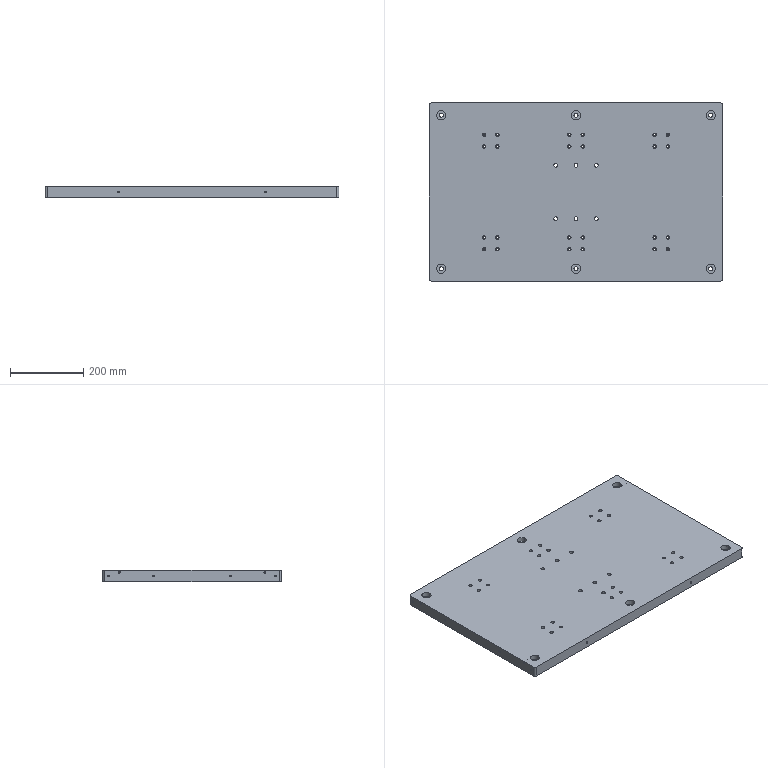NC program | Mastercam | posted with a generic post | part box 800 x 485 x 30 mm
Lines 983 to 1630 of 7047:
N9750 T5 M6
N9760 G0 G90 G17 G54 X250. Y-156. A0. S6500 M3
N9770 G43 H5 Z50. M8
N9780 Z1.
N9790 G1 Z0. F600.
N9800 X250.955 Y-155.045 F2000.
N9810 G3 X250. Y-154.09 I-.955 J0.
N9820 X248.09 Y-156. Z-.125 I0. J-1.91
N9830 X250. Y-157.91 Z-.25 I1.91 J0.
N9840 X251.91 Y-156. Z-.375 I0. J1.91
N9850 X250. Y-154.09 Z-.5 I-1.91 J0.
N9860 X248.09 Y-156. Z-.625 I0. J-1.91
N9870 X250. Y-157.91 Z-.75 I1.91 J0.
N9880 X251.91 Y-156. Z-.875 I0. J1.91
N9890 X250. Y-154.09 Z-1. I-1.91 J0.
N9900 X248.09 Y-156. Z-1.125 I0. J-1.91
N9910 X250. Y-157.91 Z-1.25 I1.91 J0.
N9920 X251.91 Y-156. Z-1.375 I0. J1.91
N9930 X250. Y-154.09 Z-1.5 I-1.91 J0.
N9940 X248.09 Y-156. Z-1.625 I0. J-1.91
N9950 X250. Y-157.91 Z-1.75 I1.91 J0.
N9960 X251.91 Y-156. Z-1.875 I0. J1.91
N9970 X250. Y-154.09 Z-2. I-1.91 J0.
N9980 X248.09 Y-156. Z-2.125 I0. J-1.91
N9990 X250. Y-157.91 Z-2.25 I1.91 J0.
N100 X251.91 Y-156. Z-2.375 I0. J1.91
N110 X250. Y-154.09 Z-2.5 I-1.91 J0.
N120 X248.09 Y-156. Z-2.625 I0. J-1.91
N130 X250. Y-157.91 Z-2.75 I1.91 J0.
N140 X251.91 Y-156. Z-2.875 I0. J1.91
N150 X250. Y-154.09 Z-3. I-1.91 J0.
N160 X248.09 Y-156. Z-3.125 I0. J-1.91
N170 X250. Y-157.91 Z-3.25 I1.91 J0.
N180 X251.91 Y-156. Z-3.375 I0. J1.91
N190 X250. Y-154.09 Z-3.5 I-1.91 J0.
N200 X248.09 Y-156. Z-3.625 I0. J-1.91
N210 X250. Y-157.91 Z-3.75 I1.91 J0.
N220 X251.91 Y-156. Z-3.875 I0. J1.91
N230 X250. Y-154.09 Z-4. I-1.91 J0.
N240 X248.09 Y-156. Z-4.125 I0. J-1.91
N250 X250. Y-157.91 Z-4.25 I1.91 J0.
N260 X251.91 Y-156. Z-4.375 I0. J1.91
N270 X250. Y-154.09 Z-4.5 I-1.91 J0.
N280 X248.09 Y-156. Z-4.625 I0. J-1.91
N290 X250. Y-157.91 Z-4.75 I1.91 J0.
N300 X251.91 Y-156. Z-4.875 I0. J1.91
N310 X250. Y-154.09 Z-5. I-1.91 J0.
N320 X248.09 Y-156. Z-5.125 I0. J-1.91
N330 X250. Y-157.91 Z-5.25 I1.91 J0.
N340 X251.91 Y-156. Z-5.375 I0. J1.91
N350 X250. Y-154.09 Z-5.5 I-1.91 J0.
N360 X248.09 Y-156. Z-5.625 I0. J-1.91
N370 X250. Y-157.91 Z-5.75 I1.91 J0.
N380 X251.91 Y-156. Z-5.875 I0. J1.91
N390 X250. Y-154.09 Z-6. I-1.91 J0.
N400 X248.09 Y-156. Z-6.125 I0. J-1.91
N410 X250. Y-157.91 Z-6.25 I1.91 J0.
N420 X251.91 Y-156. Z-6.375 I0. J1.91
N430 X250. Y-154.09 Z-6.5 I-1.91 J0.
N440 X248.09 Y-156. Z-6.625 I0. J-1.91
N450 X250. Y-157.91 Z-6.75 I1.91 J0.
N460 X251.91 Y-156. Z-6.875 I0. J1.91
N470 X250. Y-154.09 Z-7. I-1.91 J0.
N480 X248.09 Y-156. Z-7.125 I0. J-1.91
N490 X250. Y-157.91 Z-7.25 I1.91 J0.
N500 X251.91 Y-156. Z-7.375 I0. J1.91
N510 X250. Y-154.09 Z-7.5 I-1.91 J0.
N520 X248.09 Y-156. Z-7.625 I0. J-1.91
N530 X250. Y-157.91 Z-7.75 I1.91 J0.
N540 X251.91 Y-156. Z-7.875 I0. J1.91
N550 X250. Y-154.09 Z-8. I-1.91 J0.
N560 X248.09 Y-156. Z-8.125 I0. J-1.91
N570 X250. Y-157.91 Z-8.25 I1.91 J0.
N580 X251.91 Y-156. Z-8.375 I0. J1.91
N590 X250. Y-154.09 Z-8.5 I-1.91 J0.
N600 X248.09 Y-156. Z-8.625 I0. J-1.91
N610 X250. Y-157.91 Z-8.75 I1.91 J0.
N620 X251.91 Y-156. Z-8.875 I0. J1.91
N630 X250. Y-154.09 Z-9. I-1.91 J0.
N640 X248.09 Y-156. Z-9.125 I0. J-1.91
N650 X250. Y-157.91 Z-9.25 I1.91 J0.
N660 X251.91 Y-156. Z-9.375 I0. J1.91
N670 X250. Y-154.09 Z-9.5 I-1.91 J0.
N680 X248.09 Y-156. Z-9.625 I0. J-1.91
N690 X250. Y-157.91 Z-9.75 I1.91 J0.
N700 X251.91 Y-156. Z-9.875 I0. J1.91
N710 X250. Y-154.09 Z-10. I-1.91 J0.
N720 X248.09 Y-156. Z-10.125 I0. J-1.91
N730 X250. Y-157.91 Z-10.25 I1.91 J0.
N740 X251.91 Y-156. Z-10.375 I0. J1.91
N750 X250. Y-154.09 Z-10.5 I-1.91 J0.
N760 X248.09 Y-156. Z-10.625 I0. J-1.91
N770 X250. Y-157.91 Z-10.75 I1.91 J0.
N780 X251.91 Y-156. Z-10.875 I0. J1.91
N790 X250. Y-154.09 Z-11. I-1.91 J0.
N800 X248.09 Y-156. Z-11.125 I0. J-1.91
N810 X250. Y-157.91 Z-11.25 I1.91 J0.
N820 X251.91 Y-156. Z-11.375 I0. J1.91
N830 X250. Y-154.09 Z-11.5 I-1.91 J0.
N840 X248.09 Y-156. Z-11.625 I0. J-1.91
N850 X250. Y-157.91 Z-11.75 I1.91 J0.
N860 X251.91 Y-156. Z-11.875 I0. J1.91
N870 X250. Y-154.09 Z-12. I-1.91 J0.
N880 X248.09 Y-156. Z-12.125 I0. J-1.91
N890 X250. Y-157.91 Z-12.25 I1.91 J0.
N900 X251.91 Y-156. Z-12.375 I0. J1.91
N910 X250. Y-154.09 Z-12.5 I-1.91 J0.
N920 X248.09 Y-156. Z-12.625 I0. J-1.91
N930 X250. Y-157.91 Z-12.75 I1.91 J0.
N940 X251.91 Y-156. Z-12.875 I0. J1.91
N950 X250. Y-154.09 Z-13. I-1.91 J0.
N960 X248.09 Y-156. Z-13.125 I0. J-1.91
N970 X250. Y-157.91 Z-13.25 I1.91 J0.
N980 X251.91 Y-156. Z-13.375 I0. J1.91
N990 X250. Y-154.09 Z-13.5 I-1.91 J0.
N1000 X248.09 Y-156. Z-13.625 I0. J-1.91
N1010 X250. Y-157.91 Z-13.75 I1.91 J0.
N1020 X251.91 Y-156. Z-13.875 I0. J1.91
N1030 X250. Y-154.09 Z-14. I-1.91 J0.
N1040 X248.09 Y-156. I0. J-1.91 F1000.
N1050 X250. Y-157.91 I1.91 J0.
N1060 X251.91 Y-156. I0. J1.91
N1070 X250. Y-154.09 I-1.91 J0.
N1080 X249.506 Y-154.155 I0. J-1.91
N1090 X248.798 Y-155.078 I.247 J-.923
N1100 X248.83 Y-155.325 I.955 J0.
N1110 G1 X250. Y-156.
N1120 G0 Z0.
N1130 G1 X251.005 Y-154.995 F500.
N1140 G3 X250. Y-153.99 I-1.005 J0.
N1150 X247.99 Y-156. I0. J-2.01
N1160 X250. Y-158.01 I2.01 J0.
N1170 X252.01 Y-156. I0. J2.01
N1180 X250. Y-153.99 I-2.01 J0.
N1190 X249.505 Y-154.052 I0. J-2.01
N1200 X247.99 Y-156. Z-1.052 I.495 J-1.948
N1210 X250. Y-158.01 Z-2.302 I2.01 J0.
N1220 X252.01 Y-156. Z-3.552 I0. J2.01
N1230 X250. Y-153.99 Z-4.802 I-2.01 J0.
N1240 X249.505 Y-154.052 Z-5. I0. J-2.01
N1250 X247.99 Y-156. Z-6.052 I.495 J-1.948
N1260 X250. Y-158.01 Z-7.302 I2.01 J0.
N1270 X252.01 Y-156. Z-8.552 I0. J2.01
N1280 X250. Y-153.99 Z-9.802 I-2.01 J0.
N1290 X249.505 Y-154.052 Z-10. I0. J-2.01
N1300 X247.99 Y-156. Z-11.052 I.495 J-1.948
N1310 X250. Y-158.01 Z-12.302 I2.01 J0.
N1320 X252.01 Y-156. Z-13.552 I0. J2.01
N1330 X251.7 Y-154.927 Z-14. I-2.01 J0.
N1340 X250. Y-153.99 I-1.7 J-1.073
N1350 X247.99 Y-156. I0. J-2.01
N1360 X250. Y-158.01 I2.01 J0.
N1370 X252.01 Y-156. I0. J2.01
N1380 X251.7 Y-154.927 I-2.01 J0.
N1390 X251.383 Y-154.542 I-1.7 J-1.073
N1400 X250.692 Y-154.267 I-.691 J-.729
N1410 X249.963 Y-154.579 I0. J-1.004
N1420 G1 X250. Y-156.
N1430 G0 Z50.
N1440 Y-124.
N1450 Z1.
N1460 G1 Z0. F600.
N1470 X250.955 Y-123.045 F2000.
N1480 G3 X250. Y-122.09 I-.955 J0.
N1490 X248.09 Y-124. Z-.125 I0. J-1.91
N1500 X250. Y-125.91 Z-.25 I1.91 J0.
N1510 X251.91 Y-124. Z-.375 I0. J1.91
N1520 X250. Y-122.09 Z-.5 I-1.91 J0.
N1530 X248.09 Y-124. Z-.625 I0. J-1.91
N1540 X250. Y-125.91 Z-.75 I1.91 J0.
N1550 X251.91 Y-124. Z-.875 I0. J1.91
N1560 X250. Y-122.09 Z-1. I-1.91 J0.
N1570 X248.09 Y-124. Z-1.125 I0. J-1.91
N1580 X250. Y-125.91 Z-1.25 I1.91 J0.
N1590 X251.91 Y-124. Z-1.375 I0. J1.91
N1600 X250. Y-122.09 Z-1.5 I-1.91 J0.
N1610 X248.09 Y-124. Z-1.625 I0. J-1.91
N1620 X250. Y-125.91 Z-1.75 I1.91 J0.
N1630 X251.91 Y-124. Z-1.875 I0. J1.91
N1640 X250. Y-122.09 Z-2. I-1.91 J0.
N1650 X248.09 Y-124. Z-2.125 I0. J-1.91
N1660 X250. Y-125.91 Z-2.25 I1.91 J0.
N1670 X251.91 Y-124. Z-2.375 I0. J1.91
N1680 X250. Y-122.09 Z-2.5 I-1.91 J0.
N1690 X248.09 Y-124. Z-2.625 I0. J-1.91
N1700 X250. Y-125.91 Z-2.75 I1.91 J0.
N1710 X251.91 Y-124. Z-2.875 I0. J1.91
N1720 X250. Y-122.09 Z-3. I-1.91 J0.
N1730 X248.09 Y-124. Z-3.125 I0. J-1.91
N1740 X250. Y-125.91 Z-3.25 I1.91 J0.
N1750 X251.91 Y-124. Z-3.375 I0. J1.91
N1760 X250. Y-122.09 Z-3.5 I-1.91 J0.
N1770 X248.09 Y-124. Z-3.625 I0. J-1.91
N1780 X250. Y-125.91 Z-3.75 I1.91 J0.
N1790 X251.91 Y-124. Z-3.875 I0. J1.91
N1800 X250. Y-122.09 Z-4. I-1.91 J0.
N1810 X248.09 Y-124. Z-4.125 I0. J-1.91
N1820 X250. Y-125.91 Z-4.25 I1.91 J0.
N1830 X251.91 Y-124. Z-4.375 I0. J1.91
N1840 X250. Y-122.09 Z-4.5 I-1.91 J0.
N1850 X248.09 Y-124. Z-4.625 I0. J-1.91
N1860 X250. Y-125.91 Z-4.75 I1.91 J0.
N1870 X251.91 Y-124. Z-4.875 I0. J1.91
N1880 X250. Y-122.09 Z-5. I-1.91 J0.
N1890 X248.09 Y-124. Z-5.125 I0. J-1.91
N1900 X250. Y-125.91 Z-5.25 I1.91 J0.
N1910 X251.91 Y-124. Z-5.375 I0. J1.91
N1920 X250. Y-122.09 Z-5.5 I-1.91 J0.
N1930 X248.09 Y-124. Z-5.625 I0. J-1.91
N1940 X250. Y-125.91 Z-5.75 I1.91 J0.
N1950 X251.91 Y-124. Z-5.875 I0. J1.91
N1960 X250. Y-122.09 Z-6. I-1.91 J0.
N1970 X248.09 Y-124. Z-6.125 I0. J-1.91
N1980 X250. Y-125.91 Z-6.25 I1.91 J0.
N1990 X251.91 Y-124. Z-6.375 I0. J1.91
N2000 X250. Y-122.09 Z-6.5 I-1.91 J0.
N2010 X248.09 Y-124. Z-6.625 I0. J-1.91
N2020 X250. Y-125.91 Z-6.75 I1.91 J0.
N2030 X251.91 Y-124. Z-6.875 I0. J1.91
N2040 X250. Y-122.09 Z-7. I-1.91 J0.
N2050 X248.09 Y-124. Z-7.125 I0. J-1.91
N2060 X250. Y-125.91 Z-7.25 I1.91 J0.
N2070 X251.91 Y-124. Z-7.375 I0. J1.91
N2080 X250. Y-122.09 Z-7.5 I-1.91 J0.
N2090 X248.09 Y-124. Z-7.625 I0. J-1.91
N2100 X250. Y-125.91 Z-7.75 I1.91 J0.
N2110 X251.91 Y-124. Z-7.875 I0. J1.91
N2120 X250. Y-122.09 Z-8. I-1.91 J0.
N2130 X248.09 Y-124. Z-8.125 I0. J-1.91
N2140 X250. Y-125.91 Z-8.25 I1.91 J0.
N2150 X251.91 Y-124. Z-8.375 I0. J1.91
N2160 X250. Y-122.09 Z-8.5 I-1.91 J0.
N2170 X248.09 Y-124. Z-8.625 I0. J-1.91
N2180 X250. Y-125.91 Z-8.75 I1.91 J0.
N2190 X251.91 Y-124. Z-8.875 I0. J1.91
N2200 X250. Y-122.09 Z-9. I-1.91 J0.
N2210 X248.09 Y-124. Z-9.125 I0. J-1.91
N2220 X250. Y-125.91 Z-9.25 I1.91 J0.
N2230 X251.91 Y-124. Z-9.375 I0. J1.91
N2240 X250. Y-122.09 Z-9.5 I-1.91 J0.
N2250 X248.09 Y-124. Z-9.625 I0. J-1.91
N2260 X250. Y-125.91 Z-9.75 I1.91 J0.
N2270 X251.91 Y-124. Z-9.875 I0. J1.91
N2280 X250. Y-122.09 Z-10. I-1.91 J0.
N2290 X248.09 Y-124. Z-10.125 I0. J-1.91
N2300 X250. Y-125.91 Z-10.25 I1.91 J0.
N2310 X251.91 Y-124. Z-10.375 I0. J1.91
N2320 X250. Y-122.09 Z-10.5 I-1.91 J0.
N2330 X248.09 Y-124. Z-10.625 I0. J-1.91
N2340 X250. Y-125.91 Z-10.75 I1.91 J0.
N2350 X251.91 Y-124. Z-10.875 I0. J1.91
N2360 X250. Y-122.09 Z-11. I-1.91 J0.
N2370 X248.09 Y-124. Z-11.125 I0. J-1.91
N2380 X250. Y-125.91 Z-11.25 I1.91 J0.
N2390 X251.91 Y-124. Z-11.375 I0. J1.91
N2400 X250. Y-122.09 Z-11.5 I-1.91 J0.
N2410 X248.09 Y-124. Z-11.625 I0. J-1.91
N2420 X250. Y-125.91 Z-11.75 I1.91 J0.
N2430 X251.91 Y-124. Z-11.875 I0. J1.91
N2440 X250. Y-122.09 Z-12. I-1.91 J0.
N2450 X248.09 Y-124. Z-12.125 I0. J-1.91
N2460 X250. Y-125.91 Z-12.25 I1.91 J0.
N2470 X251.91 Y-124. Z-12.375 I0. J1.91
N2480 X250. Y-122.09 Z-12.5 I-1.91 J0.
N2490 X248.09 Y-124. Z-12.625 I0. J-1.91
N2500 X250. Y-125.91 Z-12.75 I1.91 J0.
N2510 X251.91 Y-124. Z-12.875 I0. J1.91
N2520 X250. Y-122.09 Z-13. I-1.91 J0.
N2530 X248.09 Y-124. Z-13.125 I0. J-1.91
N2540 X250. Y-125.91 Z-13.25 I1.91 J0.
N2550 X251.91 Y-124. Z-13.375 I0. J1.91
N2560 X250. Y-122.09 Z-13.5 I-1.91 J0.
N2570 X248.09 Y-124. Z-13.625 I0. J-1.91
N2580 X250. Y-125.91 Z-13.75 I1.91 J0.
N2590 X251.91 Y-124. Z-13.875 I0. J1.91
N2600 X250. Y-122.09 Z-14. I-1.91 J0.
N2610 X248.09 Y-124. I0. J-1.91 F1000.
N2620 X250. Y-125.91 I1.91 J0.
N2630 X251.91 Y-124. I0. J1.91
N2640 X250. Y-122.09 I-1.91 J0.
N2650 X249.506 Y-122.155 I0. J-1.91
N2660 X248.798 Y-123.078 I.247 J-.923
N2670 X248.83 Y-123.325 I.955 J0.
N2680 G1 X250. Y-124.
N2690 G0 Z0.
N2700 G1 X251.005 Y-122.995 F500.
N2710 G3 X250. Y-121.99 I-1.005 J0.
N2720 X247.99 Y-124. I0. J-2.01
N2730 X250. Y-126.01 I2.01 J0.
N2740 X252.01 Y-124. I0. J2.01
N2750 X250. Y-121.99 I-2.01 J0.
N2760 X249.505 Y-122.052 I0. J-2.01
N2770 X247.99 Y-124. Z-1.052 I.495 J-1.948
N2780 X250. Y-126.01 Z-2.302 I2.01 J0.
N2790 X252.01 Y-124. Z-3.552 I0. J2.01
N2800 X250. Y-121.99 Z-4.802 I-2.01 J0.
N2810 X249.505 Y-122.052 Z-5. I0. J-2.01
N2820 X247.99 Y-124. Z-6.052 I.495 J-1.948
N2830 X250. Y-126.01 Z-7.302 I2.01 J0.
N2840 X252.01 Y-124. Z-8.552 I0. J2.01
N2850 X250. Y-121.99 Z-9.802 I-2.01 J0.
N2860 X249.505 Y-122.052 Z-10. I0. J-2.01
N2870 X247.99 Y-124. Z-11.052 I.495 J-1.948
N2880 X250. Y-126.01 Z-12.302 I2.01 J0.
N2890 X252.01 Y-124. Z-13.552 I0. J2.01
N2900 X251.7 Y-122.927 Z-14. I-2.01 J0.
N2910 X250. Y-121.99 I-1.7 J-1.073
N2920 X247.99 Y-124. I0. J-2.01
N2930 X250. Y-126.01 I2.01 J0.
N2940 X252.01 Y-124. I0. J2.01
N2950 X251.7 Y-122.927 I-2.01 J0.
N2960 X251.383 Y-122.542 I-1.7 J-1.073
N2970 X250.692 Y-122.267 I-.691 J-.729
N2980 X249.963 Y-122.579 I0. J-1.004
N2990 G1 X250. Y-124.
N3000 G0 Z50.
N3010 X214.
N3020 Z1.
N3030 G1 Z0. F600.
N3040 X214.955 Y-123.045 F2000.
N3050 G3 X214. Y-122.09 I-.955 J0.
N3060 X212.09 Y-124. Z-.125 I0. J-1.91
N3070 X214. Y-125.91 Z-.25 I1.91 J0.
N3080 X215.91 Y-124. Z-.375 I0. J1.91
N3090 X214. Y-122.09 Z-.5 I-1.91 J0.
N3100 X212.09 Y-124. Z-.625 I0. J-1.91
N3110 X214. Y-125.91 Z-.75 I1.91 J0.
N3120 X215.91 Y-124. Z-.875 I0. J1.91
N3130 X214. Y-122.09 Z-1. I-1.91 J0.
N3140 X212.09 Y-124. Z-1.125 I0. J-1.91
N3150 X214. Y-125.91 Z-1.25 I1.91 J0.
N3160 X215.91 Y-124. Z-1.375 I0. J1.91
N3170 X214. Y-122.09 Z-1.5 I-1.91 J0.
N3180 X212.09 Y-124. Z-1.625 I0. J-1.91
N3190 X214. Y-125.91 Z-1.75 I1.91 J0.
N3200 X215.91 Y-124. Z-1.875 I0. J1.91
N3210 X214. Y-122.09 Z-2. I-1.91 J0.
N3220 X212.09 Y-124. Z-2.125 I0. J-1.91
N3230 X214. Y-125.91 Z-2.25 I1.91 J0.
N3240 X215.91 Y-124. Z-2.375 I0. J1.91
N3250 X214. Y-122.09 Z-2.5 I-1.91 J0.
N3260 X212.09 Y-124. Z-2.625 I0. J-1.91
N3270 X214. Y-125.91 Z-2.75 I1.91 J0.
N3280 X215.91 Y-124. Z-2.875 I0. J1.91
N3290 X214. Y-122.09 Z-3. I-1.91 J0.
N3300 X212.09 Y-124. Z-3.125 I0. J-1.91
N3310 X214. Y-125.91 Z-3.25 I1.91 J0.
N3320 X215.91 Y-124. Z-3.375 I0. J1.91
N3330 X214. Y-122.09 Z-3.5 I-1.91 J0.
N3340 X212.09 Y-124. Z-3.625 I0. J-1.91
N3350 X214. Y-125.91 Z-3.75 I1.91 J0.
N3360 X215.91 Y-124. Z-3.875 I0. J1.91
N3370 X214. Y-122.09 Z-4. I-1.91 J0.
N3380 X212.09 Y-124. Z-4.125 I0. J-1.91
N3390 X214. Y-125.91 Z-4.25 I1.91 J0.
N3400 X215.91 Y-124. Z-4.375 I0. J1.91
N3410 X214. Y-122.09 Z-4.5 I-1.91 J0.
N3420 X212.09 Y-124. Z-4.625 I0. J-1.91
N3430 X214. Y-125.91 Z-4.75 I1.91 J0.
N3440 X215.91 Y-124. Z-4.875 I0. J1.91
N3450 X214. Y-122.09 Z-5. I-1.91 J0.
N3460 X212.09 Y-124. Z-5.125 I0. J-1.91
N3470 X214. Y-125.91 Z-5.25 I1.91 J0.
N3480 X215.91 Y-124. Z-5.375 I0. J1.91
N3490 X214. Y-122.09 Z-5.5 I-1.91 J0.
N3500 X212.09 Y-124. Z-5.625 I0. J-1.91
N3510 X214. Y-125.91 Z-5.75 I1.91 J0.
N3520 X215.91 Y-124. Z-5.875 I0. J1.91
N3530 X214. Y-122.09 Z-6. I-1.91 J0.
N3540 X212.09 Y-124. Z-6.125 I0. J-1.91
N3550 X214. Y-125.91 Z-6.25 I1.91 J0.
N3560 X215.91 Y-124. Z-6.375 I0. J1.91
N3570 X214. Y-122.09 Z-6.5 I-1.91 J0.
N3580 X212.09 Y-124. Z-6.625 I0. J-1.91
N3590 X214. Y-125.91 Z-6.75 I1.91 J0.
N3600 X215.91 Y-124. Z-6.875 I0. J1.91
N3610 X214. Y-122.09 Z-7. I-1.91 J0.
N3620 X212.09 Y-124. Z-7.125 I0. J-1.91
N3630 X214. Y-125.91 Z-7.25 I1.91 J0.
N3640 X215.91 Y-124. Z-7.375 I0. J1.91
N3650 X214. Y-122.09 Z-7.5 I-1.91 J0.
N3660 X212.09 Y-124. Z-7.625 I0. J-1.91
N3670 X214. Y-125.91 Z-7.75 I1.91 J0.
N3680 X215.91 Y-124. Z-7.875 I0. J1.91
N3690 X214. Y-122.09 Z-8. I-1.91 J0.
N3700 X212.09 Y-124. Z-8.125 I0. J-1.91
N3710 X214. Y-125.91 Z-8.25 I1.91 J0.
N3720 X215.91 Y-124. Z-8.375 I0. J1.91
N3730 X214. Y-122.09 Z-8.5 I-1.91 J0.
N3740 X212.09 Y-124. Z-8.625 I0. J-1.91
N3750 X214. Y-125.91 Z-8.75 I1.91 J0.
N3760 X215.91 Y-124. Z-8.875 I0. J1.91
N3770 X214. Y-122.09 Z-9. I-1.91 J0.
N3780 X212.09 Y-124. Z-9.125 I0. J-1.91
N3790 X214. Y-125.91 Z-9.25 I1.91 J0.
N3800 X215.91 Y-124. Z-9.375 I0. J1.91
N3810 X214. Y-122.09 Z-9.5 I-1.91 J0.
N3820 X212.09 Y-124. Z-9.625 I0. J-1.91
N3830 X214. Y-125.91 Z-9.75 I1.91 J0.
N3840 X215.91 Y-124. Z-9.875 I0. J1.91
N3850 X214. Y-122.09 Z-10. I-1.91 J0.
N3860 X212.09 Y-124. Z-10.125 I0. J-1.91
N3870 X214. Y-125.91 Z-10.25 I1.91 J0.
N3880 X215.91 Y-124. Z-10.375 I0. J1.91
N3890 X214. Y-122.09 Z-10.5 I-1.91 J0.
N3900 X212.09 Y-124. Z-10.625 I0. J-1.91
N3910 X214. Y-125.91 Z-10.75 I1.91 J0.
N3920 X215.91 Y-124. Z-10.875 I0. J1.91
N3930 X214. Y-122.09 Z-11. I-1.91 J0.
N3940 X212.09 Y-124. Z-11.125 I0. J-1.91
N3950 X214. Y-125.91 Z-11.25 I1.91 J0.
N3960 X215.91 Y-124. Z-11.375 I0. J1.91
N3970 X214. Y-122.09 Z-11.5 I-1.91 J0.
N3980 X212.09 Y-124. Z-11.625 I0. J-1.91
N3990 X214. Y-125.91 Z-11.75 I1.91 J0.
N4000 X215.91 Y-124. Z-11.875 I0. J1.91
N4010 X214. Y-122.09 Z-12. I-1.91 J0.
N4020 X212.09 Y-124. Z-12.125 I0. J-1.91
N4030 X214. Y-125.91 Z-12.25 I1.91 J0.
N4040 X215.91 Y-124. Z-12.375 I0. J1.91
N4050 X214. Y-122.09 Z-12.5 I-1.91 J0.
N4060 X212.09 Y-124. Z-12.625 I0. J-1.91
N4070 X214. Y-125.91 Z-12.75 I1.91 J0.
N4080 X215.91 Y-124. Z-12.875 I0. J1.91
N4090 X214. Y-122.09 Z-13. I-1.91 J0.
N4100 X212.09 Y-124. Z-13.125 I0. J-1.91
N4110 X214. Y-125.91 Z-13.25 I1.91 J0.
N4120 X215.91 Y-124. Z-13.375 I0. J1.91
N4130 X214. Y-122.09 Z-13.5 I-1.91 J0.
N4140 X212.09 Y-124. Z-13.625 I0. J-1.91
N4150 X214. Y-125.91 Z-13.75 I1.91 J0.
N4160 X215.91 Y-124. Z-13.875 I0. J1.91
N4170 X214. Y-122.09 Z-14. I-1.91 J0.
N4180 X212.09 Y-124. I0. J-1.91 F1000.
N4190 X214. Y-125.91 I1.91 J0.
N4200 X215.91 Y-124. I0. J1.91
N4210 X214. Y-122.09 I-1.91 J0.
N4220 X213.506 Y-122.155 I0. J-1.91
N4230 X212.798 Y-123.078 I.247 J-.923
N4240 X212.83 Y-123.325 I.955 J0.
N4250 G1 X214. Y-124.
N4260 G0 Z0.
N4270 G1 X215.005 Y-122.995 F500.
N4280 G3 X214. Y-121.99 I-1.005 J0.
N4290 X211.99 Y-124. I0. J-2.01
N4300 X214. Y-126.01 I2.01 J0.
N4310 X216.01 Y-124. I0. J2.01
N4320 X214. Y-121.99 I-2.01 J0.
N4330 X213.505 Y-122.052 I0. J-2.01
N4340 X211.99 Y-124. Z-1.052 I.495 J-1.948
N4350 X214. Y-126.01 Z-2.302 I2.01 J0.
N4360 X216.01 Y-124. Z-3.552 I0. J2.01
N4370 X214. Y-121.99 Z-4.802 I-2.01 J0.
N4380 X213.505 Y-122.052 Z-5. I0. J-2.01
N4390 X211.99 Y-124. Z-6.052 I.495 J-1.948
N4400 X214. Y-126.01 Z-7.302 I2.01 J0.
N4410 X216.01 Y-124. Z-8.552 I0. J2.01
N4420 X214. Y-121.99 Z-9.802 I-2.01 J0.
N4430 X213.505 Y-122.052 Z-10. I0. J-2.01
N4440 X211.99 Y-124. Z-11.052 I.495 J-1.948
N4450 X214. Y-126.01 Z-12.302 I2.01 J0.
N4460 X216.01 Y-124. Z-13.552 I0. J2.01
N4470 X215.7 Y-122.927 Z-14. I-2.01 J0.
N4480 X214. Y-121.99 I-1.7 J-1.073
N4490 X211.99 Y-124. I0. J-2.01
N4500 X214. Y-126.01 I2.01 J0.
N4510 X216.01 Y-124. I0. J2.01
N4520 X215.7 Y-122.927 I-2.01 J0.
N4530 X215.383 Y-122.542 I-1.7 J-1.073
N4540 X214.692 Y-122.267 I-.691 J-.729
N4550 X213.963 Y-122.579 I0. J-1.004
N4560 G1 X214. Y-124.
N4570 G0 Z50.
N4580 Y-156.
N4590 Z1.
N4600 G1 Z0. F600.
N4610 X214.955 Y-155.045 F2000.
N4620 G3 X214. Y-154.09 I-.955 J0.
N4630 X212.09 Y-156. Z-.125 I0. J-1.91
N4640 X214. Y-157.91 Z-.25 I1.91 J0.
N4650 X215.91 Y-156. Z-.375 I0. J1.91
N4660 X214. Y-154.09 Z-.5 I-1.91 J0.
N4670 X212.09 Y-156. Z-.625 I0. J-1.91
N4680 X214. Y-157.91 Z-.75 I1.91 J0.
N4690 X215.91 Y-156. Z-.875 I0. J1.91
N4700 X214. Y-154.09 Z-1. I-1.91 J0.
N4710 X212.09 Y-156. Z-1.125 I0. J-1.91
N4720 X214. Y-157.91 Z-1.25 I1.91 J0.
N4730 X215.91 Y-156. Z-1.375 I0. J1.91
N4740 X214. Y-154.09 Z-1.5 I-1.91 J0.
N4750 X212.09 Y-156. Z-1.625 I0. J-1.91
N4760 X214. Y-157.91 Z-1.75 I1.91 J0.
N4770 X215.91 Y-156. Z-1.875 I0. J1.91
N4780 X214. Y-154.09 Z-2. I-1.91 J0.
N4790 X212.09 Y-156. Z-2.125 I0. J-1.91
N4800 X214. Y-157.91 Z-2.25 I1.91 J0.
N4810 X215.91 Y-156. Z-2.375 I0. J1.91
N4820 X214. Y-154.09 Z-2.5 I-1.91 J0.
N4830 X212.09 Y-156. Z-2.625 I0. J-1.91
N4840 X214. Y-157.91 Z-2.75 I1.91 J0.
N4850 X215.91 Y-156. Z-2.875 I0. J1.91
N4860 X214. Y-154.09 Z-3. I-1.91 J0.
N4870 X212.09 Y-156. Z-3.125 I0. J-1.91
N4880 X214. Y-157.91 Z-3.25 I1.91 J0.
N4890 X215.91 Y-156. Z-3.375 I0. J1.91
N4900 X214. Y-154.09 Z-3.5 I-1.91 J0.
N4910 X212.09 Y-156. Z-3.625 I0. J-1.91
N4920 X214. Y-157.91 Z-3.75 I1.91 J0.
N4930 X215.91 Y-156. Z-3.875 I0. J1.91
N4940 X214. Y-154.09 Z-4. I-1.91 J0.
N4950 X212.09 Y-156. Z-4.125 I0. J-1.91
N4960 X214. Y-157.91 Z-4.25 I1.91 J0.
N4970 X215.91 Y-156. Z-4.375 I0. J1.91
N4980 X214. Y-154.09 Z-4.5 I-1.91 J0.
N4990 X212.09 Y-156. Z-4.625 I0. J-1.91
N5000 X214. Y-157.91 Z-4.75 I1.91 J0.
N5010 X215.91 Y-156. Z-4.875 I0. J1.91
N5020 X214. Y-154.09 Z-5. I-1.91 J0.
N5030 X212.09 Y-156. Z-5.125 I0. J-1.91
N5040 X214. Y-157.91 Z-5.25 I1.91 J0.
N5050 X215.91 Y-156. Z-5.375 I0. J1.91
N5060 X214. Y-154.09 Z-5.5 I-1.91 J0.
N5070 X212.09 Y-156. Z-5.625 I0. J-1.91
N5080 X214. Y-157.91 Z-5.75 I1.91 J0.
N5090 X215.91 Y-156. Z-5.875 I0. J1.91
N5100 X214. Y-154.09 Z-6. I-1.91 J0.
N5110 X212.09 Y-156. Z-6.125 I0. J-1.91
N5120 X214. Y-157.91 Z-6.25 I1.91 J0.
N5130 X215.91 Y-156. Z-6.375 I0. J1.91
N5140 X214. Y-154.09 Z-6.5 I-1.91 J0.
N5150 X212.09 Y-156. Z-6.625 I0. J-1.91
N5160 X214. Y-157.91 Z-6.75 I1.91 J0.
N5170 X215.91 Y-156. Z-6.875 I0. J1.91
N5180 X214. Y-154.09 Z-7. I-1.91 J0.
N5190 X212.09 Y-156. Z-7.125 I0. J-1.91
N5200 X214. Y-157.91 Z-7.25 I1.91 J0.
N5210 X215.91 Y-156. Z-7.375 I0. J1.91
N5220 X214. Y-154.09 Z-7.5 I-1.91 J0.
N5230 X212.09 Y-156. Z-7.625 I0. J-1.91
N5240 X214. Y-157.91 Z-7.75 I1.91 J0.
N5250 X215.91 Y-156. Z-7.875 I0. J1.91
N5260 X214. Y-154.09 Z-8. I-1.91 J0.
N5270 X212.09 Y-156. Z-8.125 I0. J-1.91
N5280 X214. Y-157.91 Z-8.25 I1.91 J0.
N5290 X215.91 Y-156. Z-8.375 I0. J1.91
N5300 X214. Y-154.09 Z-8.5 I-1.91 J0.
N5310 X212.09 Y-156. Z-8.625 I0. J-1.91
N5320 X214. Y-157.91 Z-8.75 I1.91 J0.
N5330 X215.91 Y-156. Z-8.875 I0. J1.91
N5340 X214. Y-154.09 Z-9. I-1.91 J0.
N5350 X212.09 Y-156. Z-9.125 I0. J-1.91
N5360 X214. Y-157.91 Z-9.25 I1.91 J0.
N5370 X215.91 Y-156. Z-9.375 I0. J1.91
N5380 X214. Y-154.09 Z-9.5 I-1.91 J0.
N5390 X212.09 Y-156. Z-9.625 I0. J-1.91
N5400 X214. Y-157.91 Z-9.75 I1.91 J0.
N5410 X215.91 Y-156. Z-9.875 I0. J1.91
N5420 X214. Y-154.09 Z-10. I-1.91 J0.
N5430 X212.09 Y-156. Z-10.125 I0. J-1.91
N5440 X214. Y-157.91 Z-10.25 I1.91 J0.
N5450 X215.91 Y-156. Z-10.375 I0. J1.91
N5460 X214. Y-154.09 Z-10.5 I-1.91 J0.
N5470 X212.09 Y-156. Z-10.625 I0. J-1.91
N5480 X214. Y-157.91 Z-10.75 I1.91 J0.
N5490 X215.91 Y-156. Z-10.875 I0. J1.91
N5500 X214. Y-154.09 Z-11. I-1.91 J0.
N5510 X212.09 Y-156. Z-11.125 I0. J-1.91
N5520 X214. Y-157.91 Z-11.25 I1.91 J0.
N5530 X215.91 Y-156. Z-11.375 I0. J1.91
N5540 X214. Y-154.09 Z-11.5 I-1.91 J0.
N5550 X212.09 Y-156. Z-11.625 I0. J-1.91
N5560 X214. Y-157.91 Z-11.75 I1.91 J0.
N5570 X215.91 Y-156. Z-11.875 I0. J1.91
N5580 X214. Y-154.09 Z-12. I-1.91 J0.
N5590 X212.09 Y-156. Z-12.125 I0. J-1.91
N5600 X214. Y-157.91 Z-12.25 I1.91 J0.
N5610 X215.91 Y-156. Z-12.375 I0. J1.91
N5620 X214. Y-154.09 Z-12.5 I-1.91 J0.
N5630 X212.09 Y-156. Z-12.625 I0. J-1.91
N5640 X214. Y-157.91 Z-12.75 I1.91 J0.
N5650 X215.91 Y-156. Z-12.875 I0. J1.91
N5660 X214. Y-154.09 Z-13. I-1.91 J0.
N5670 X212.09 Y-156. Z-13.125 I0. J-1.91
N5680 X214. Y-157.91 Z-13.25 I1.91 J0.
N5690 X215.91 Y-156. Z-13.375 I0. J1.91
N5700 X214. Y-154.09 Z-13.5 I-1.91 J0.
N5710 X212.09 Y-156. Z-13.625 I0. J-1.91
N5720 X214. Y-157.91 Z-13.75 I1.91 J0.
N5730 X215.91 Y-156. Z-13.875 I0. J1.91
N5740 X214. Y-154.09 Z-14. I-1.91 J0.
N5750 X212.09 Y-156. I0. J-1.91 F1000.
N5760 X214. Y-157.91 I1.91 J0.
N5770 X215.91 Y-156. I0. J1.91
N5780 X214. Y-154.09 I-1.91 J0.
N5790 X213.506 Y-154.155 I0. J-1.91
N5800 X212.798 Y-155.078 I.247 J-.923
N5810 X212.83 Y-155.325 I.955 J0.
N5820 G1 X214. Y-156.
N5830 G0 Z0.
N5840 G1 X215.005 Y-154.995 F500.
N5850 G3 X214. Y-153.99 I-1.005 J0.
N5860 X211.99 Y-156. I0. J-2.01
N5870 X214. Y-158.01 I2.01 J0.
N5880 X216.01 Y-156. I0. J2.01
N5890 X214. Y-153.99 I-2.01 J0.
N5900 X213.505 Y-154.052 I0. J-2.01
N5910 X211.99 Y-156. Z-1.052 I.495 J-1.948
N5920 X214. Y-158.01 Z-2.302 I2.01 J0.
N5930 X216.01 Y-156. Z-3.552 I0. J2.01
N5940 X214. Y-153.99 Z-4.802 I-2.01 J0.
N5950 X213.505 Y-154.052 Z-5. I0. J-2.01
N5960 X211.99 Y-156. Z-6.052 I.495 J-1.948
N5970 X214. Y-158.01 Z-7.302 I2.01 J0.
N5980 X216.01 Y-156. Z-8.552 I0. J2.01
N5990 X214. Y-153.99 Z-9.802 I-2.01 J0.
N6000 X213.505 Y-154.052 Z-10. I0. J-2.01
N6010 X211.99 Y-156. Z-11.052 I.495 J-1.948
N6020 X214. Y-158.01 Z-12.302 I2.01 J0.
N6030 X216.01 Y-156. Z-13.552 I0. J2.01
N6040 X215.7 Y-154.927 Z-14. I-2.01 J0.
N6050 X214. Y-153.99 I-1.7 J-1.073
N6060 X211.99 Y-156. I0. J-2.01
N6070 X214. Y-158.01 I2.01 J0.
N6080 X216.01 Y-156. I0. J2.01
N6090 X215.7 Y-154.927 I-2.01 J0.
N6100 X215.383 Y-154.542 I-1.7 J-1.073
N6110 X214.692 Y-154.267 I-.691 J-.729
N6120 X213.963 Y-154.579 I0. J-1.004
N6130 G1 X214. Y-156.
N6140 G0 Z50.
N6150 X18.
N6160 Z1.
N6170 G1 Z0. F600.
N6180 X18.955 Y-155.045 F2000.
N6190 G3 X18. Y-154.09 I-.955 J0.
N6200 X16.09 Y-156. Z-.125 I0. J-1.91
N6210 X18. Y-157.91 Z-.25 I1.91 J0.
N6220 X19.91 Y-156. Z-.375 I0. J1.91
N6230 X18. Y-154.09 Z-.5 I-1.91 J0.
N6240 X16.09 Y-156. Z-.625 I0. J-1.91
N6250 X18. Y-157.91 Z-.75 I1.91 J0.
N6260 X19.91 Y-156. Z-.875 I0. J1.91
N6270 X18. Y-154.09 Z-1. I-1.91 J0.
N6280 X16.09 Y-156. Z-1.125 I0. J-1.91
N6290 X18. Y-157.91 Z-1.25 I1.91 J0.
N6300 X19.91 Y-156. Z-1.375 I0. J1.91
N6310 X18. Y-154.09 Z-1.5 I-1.91 J0.
N6320 X16.09 Y-156. Z-1.625 I0. J-1.91